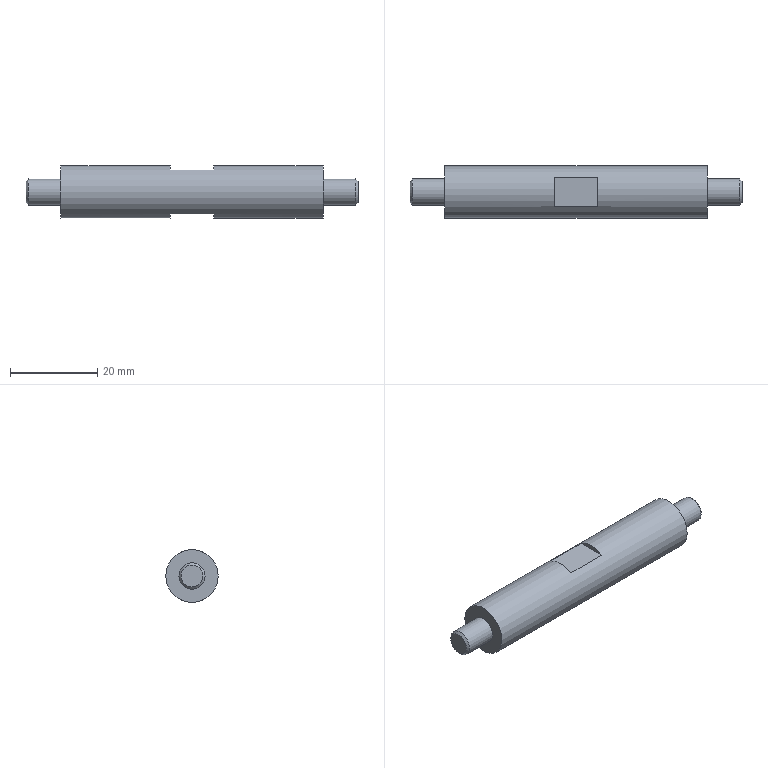Part | NX | features BREP 1 | 1 solid | 15 faces | box 76 x 12 x 12 mm | volume 7144 mm3 | plane 10 | cylinder 3 | cone 2 | commonest cylinder face diameters 6 x2 12 x1
STEP:
#1=CARTESIAN_POINT('',(30.,-6.,0.));
#2=VERTEX_POINT('',#1);
#3=CARTESIAN_POINT('',(30.,0.,0.));
#4=DIRECTION('',(-1.,0.,0.));
#5=DIRECTION('',(0.,-1.,0.));
#6=AXIS2_PLACEMENT_3D('',#3,#4,#5);
#7=CIRCLE('',#6,6.);
#8=EDGE_CURVE('',#2,#2,#7,.T.);
#9=ORIENTED_EDGE('',*,*,#8,.T.);
#10=EDGE_LOOP('',(#9));
#11=FACE_BOUND('',#10,.T.);
#12=CARTESIAN_POINT('',(-5.,-3.317,-5.));
#13=VERTEX_POINT('',#12);
#14=CARTESIAN_POINT('',(5.,-3.317,-5.));
#15=VERTEX_POINT('',#14);
#16=CARTESIAN_POINT('',(-38.,-3.317,-5.));
#17=DIRECTION('',(1.,0.,0.));
#18=VECTOR('',#17,1000.);
#19=LINE('',#16,#18);
#20=EDGE_CURVE('',#13,#15,#19,.T.);
#21=ORIENTED_EDGE('',*,*,#20,.T.);
#22=CARTESIAN_POINT('',(5.,3.317,-5.));
#23=VERTEX_POINT('',#22);
#24=CARTESIAN_POINT('',(5.,0.,0.));
#25=DIRECTION('',(1.,0.,0.));
#26=DIRECTION('',(0.,-1.,0.));
#27=AXIS2_PLACEMENT_3D('',#24,#25,#26);
#28=CIRCLE('',#27,6.);
#29=EDGE_CURVE('',#15,#23,#28,.T.);
#30=ORIENTED_EDGE('',*,*,#29,.T.);
#31=CARTESIAN_POINT('',(-5.,3.317,-5.));
#32=VERTEX_POINT('',#31);
#33=CARTESIAN_POINT('',(-38.,3.317,-5.));
#34=DIRECTION('',(-1.,0.,0.));
#35=VECTOR('',#34,1000.);
#36=LINE('',#33,#35);
#37=EDGE_CURVE('',#23,#32,#36,.T.);
#38=ORIENTED_EDGE('',*,*,#37,.T.);
#39=CARTESIAN_POINT('',(-5.,0.,0.));
#40=DIRECTION('',(-1.,0.,0.));
#41=DIRECTION('',(0.,-1.,0.));
#42=AXIS2_PLACEMENT_3D('',#39,#40,#41);
#43=CIRCLE('',#42,6.);
#44=EDGE_CURVE('',#32,#13,#43,.T.);
#45=ORIENTED_EDGE('',*,*,#44,.T.);
#46=EDGE_LOOP('',(#21,#30,#38,#45));
#47=FACE_BOUND('',#46,.T.);
#48=CARTESIAN_POINT('',(-30.,-6.,0.));
#49=VERTEX_POINT('',#48);
#50=CARTESIAN_POINT('',(-30.,0.,0.));
#51=DIRECTION('',(1.,0.,0.));
#52=DIRECTION('',(0.,-1.,0.));
#53=AXIS2_PLACEMENT_3D('',#50,#51,#52);
#54=CIRCLE('',#53,6.);
#55=EDGE_CURVE('',#49,#49,#54,.T.);
#56=ORIENTED_EDGE('',*,*,#55,.T.);
#57=EDGE_LOOP('',(#56));
#58=FACE_BOUND('',#57,.T.);
#59=CARTESIAN_POINT('',(5.,3.317,5.));
#60=VERTEX_POINT('',#59);
#61=CARTESIAN_POINT('',(5.,-3.317,5.));
#62=VERTEX_POINT('',#61);
#63=CARTESIAN_POINT('',(5.,0.,0.));
#64=DIRECTION('',(1.,0.,0.));
#65=DIRECTION('',(0.,-1.,0.));
#66=AXIS2_PLACEMENT_3D('',#63,#64,#65);
#67=CIRCLE('',#66,6.);
#68=EDGE_CURVE('',#60,#62,#67,.T.);
#69=ORIENTED_EDGE('',*,*,#68,.T.);
#70=CARTESIAN_POINT('',(-5.,-3.317,5.));
#71=VERTEX_POINT('',#70);
#72=CARTESIAN_POINT('',(-38.,-3.317,5.));
#73=DIRECTION('',(-1.,0.,0.));
#74=VECTOR('',#73,1000.);
#75=LINE('',#72,#74);
#76=EDGE_CURVE('',#62,#71,#75,.T.);
#77=ORIENTED_EDGE('',*,*,#76,.T.);
#78=CARTESIAN_POINT('',(-5.,3.317,5.));
#79=VERTEX_POINT('',#78);
#80=CARTESIAN_POINT('',(-5.,0.,0.));
#81=DIRECTION('',(-1.,0.,0.));
#82=DIRECTION('',(0.,-1.,0.));
#83=AXIS2_PLACEMENT_3D('',#80,#81,#82);
#84=CIRCLE('',#83,6.);
#85=EDGE_CURVE('',#71,#79,#84,.T.);
#86=ORIENTED_EDGE('',*,*,#85,.T.);
#87=CARTESIAN_POINT('',(-38.,3.317,5.));
#88=DIRECTION('',(1.,0.,0.));
#89=VECTOR('',#88,1000.);
#90=LINE('',#87,#89);
#91=EDGE_CURVE('',#79,#60,#90,.T.);
#92=ORIENTED_EDGE('',*,*,#91,.T.);
#93=EDGE_LOOP('',(#69,#77,#86,#92));
#94=FACE_BOUND('',#93,.T.);
#95=CARTESIAN_POINT('',(-38.,0.,0.));
#96=DIRECTION('',(-1.,0.,0.));
#97=DIRECTION('',(0.,1.,0.));
#98=AXIS2_PLACEMENT_3D('',#95,#96,#97);
#99=CYLINDRICAL_SURFACE('',#98,6.);
#100=ADVANCED_FACE('',(#11,#47,#58,#94),#99,.T.);
#101=ORIENTED_EDGE('',*,*,#29,.F.);
#102=CARTESIAN_POINT('',(5.,0.,-5.));
#103=DIRECTION('',(0.,1.,0.));
#104=VECTOR('',#103,1000.);
#105=LINE('',#102,#104);
#106=EDGE_CURVE('',#15,#23,#105,.T.);
#107=ORIENTED_EDGE('',*,*,#106,.T.);
#108=EDGE_LOOP('',(#101,#107));
#109=FACE_BOUND('',#108,.T.);
#110=CARTESIAN_POINT('',(5.,0.,0.));
#111=DIRECTION('',(-1.,0.,0.));
#112=DIRECTION('',(0.,0.,-1.));
#113=AXIS2_PLACEMENT_3D('',#110,#111,#112);
#114=PLANE('',#113);
#115=ADVANCED_FACE('',(#109),#114,.T.);
#116=ORIENTED_EDGE('',*,*,#20,.F.);
#117=CARTESIAN_POINT('',(-5.,6.286,-5.));
#118=DIRECTION('',(0.,-1.,0.));
#119=VECTOR('',#118,1000.);
#120=LINE('',#117,#119);
#121=EDGE_CURVE('',#32,#13,#120,.T.);
#122=ORIENTED_EDGE('',*,*,#121,.F.);
#123=ORIENTED_EDGE('',*,*,#37,.F.);
#124=ORIENTED_EDGE('',*,*,#106,.F.);
#125=EDGE_LOOP('',(#116,#122,#123,#124));
#126=FACE_BOUND('',#125,.T.);
#127=CARTESIAN_POINT('',(-5.,6.286,-5.));
#128=DIRECTION('',(0.,0.,1.));
#129=DIRECTION('',(-1.,0.,0.));
#130=AXIS2_PLACEMENT_3D('',#127,#128,#129);
#131=PLANE('',#130);
#132=ADVANCED_FACE('',(#126),#131,.F.);
#133=ORIENTED_EDGE('',*,*,#44,.F.);
#134=ORIENTED_EDGE('',*,*,#121,.T.);
#135=EDGE_LOOP('',(#133,#134));
#136=FACE_BOUND('',#135,.T.);
#137=CARTESIAN_POINT('',(-5.,0.,0.));
#138=DIRECTION('',(-1.,0.,0.));
#139=DIRECTION('',(0.,0.,-1.));
#140=AXIS2_PLACEMENT_3D('',#137,#138,#139);
#141=PLANE('',#140);
#142=ADVANCED_FACE('',(#136),#141,.F.);
#143=ORIENTED_EDGE('',*,*,#55,.F.);
#144=EDGE_LOOP('',(#143));
#145=FACE_BOUND('',#144,.T.);
#146=CARTESIAN_POINT('',(-30.,-3.,0.));
#147=VERTEX_POINT('',#146);
#148=CARTESIAN_POINT('',(-30.,0.,0.));
#149=DIRECTION('',(-1.,0.,0.));
#150=DIRECTION('',(0.,-1.,0.));
#151=AXIS2_PLACEMENT_3D('',#148,#149,#150);
#152=CIRCLE('',#151,3.);
#153=EDGE_CURVE('',#147,#147,#152,.T.);
#154=ORIENTED_EDGE('',*,*,#153,.F.);
#155=EDGE_LOOP('',(#154));
#156=FACE_BOUND('',#155,.T.);
#157=CARTESIAN_POINT('',(-30.,6.,0.));
#158=DIRECTION('',(1.,0.,0.));
#159=DIRECTION('',(0.,-1.,0.));
#160=AXIS2_PLACEMENT_3D('',#157,#158,#159);
#161=PLANE('',#160);
#162=ADVANCED_FACE('',(#145,#156),#161,.F.);
#163=CARTESIAN_POINT('',(30.,-3.,0.));
#164=VERTEX_POINT('',#163);
#165=CARTESIAN_POINT('',(30.,0.,0.));
#166=DIRECTION('',(1.,0.,0.));
#167=DIRECTION('',(0.,-1.,0.));
#168=AXIS2_PLACEMENT_3D('',#165,#166,#167);
#169=CIRCLE('',#168,3.);
#170=EDGE_CURVE('',#164,#164,#169,.T.);
#171=ORIENTED_EDGE('',*,*,#170,.F.);
#172=EDGE_LOOP('',(#171));
#173=FACE_BOUND('',#172,.T.);
#174=ORIENTED_EDGE('',*,*,#8,.F.);
#175=EDGE_LOOP('',(#174));
#176=FACE_BOUND('',#175,.T.);
#177=CARTESIAN_POINT('',(30.,3.,0.));
#178=DIRECTION('',(-1.,0.,0.));
#179=DIRECTION('',(0.,1.,0.));
#180=AXIS2_PLACEMENT_3D('',#177,#178,#179);
#181=PLANE('',#180);
#182=ADVANCED_FACE('',(#173,#176),#181,.F.);
#183=CARTESIAN_POINT('',(-37.5,-3.,0.));
#184=VERTEX_POINT('',#183);
#185=CARTESIAN_POINT('',(-37.5,0.,0.));
#186=DIRECTION('',(1.,0.,0.));
#187=DIRECTION('',(0.,-1.,0.));
#188=AXIS2_PLACEMENT_3D('',#185,#186,#187);
#189=CIRCLE('',#188,3.);
#190=EDGE_CURVE('',#184,#184,#189,.T.);
#191=ORIENTED_EDGE('',*,*,#190,.T.);
#192=EDGE_LOOP('',(#191));
#193=FACE_BOUND('',#192,.T.);
#194=ORIENTED_EDGE('',*,*,#153,.T.);
#195=EDGE_LOOP('',(#194));
#196=FACE_BOUND('',#195,.T.);
#197=CARTESIAN_POINT('',(-38.,0.,0.));
#198=DIRECTION('',(-1.,0.,0.));
#199=DIRECTION('',(0.,1.,0.));
#200=AXIS2_PLACEMENT_3D('',#197,#198,#199);
#201=CYLINDRICAL_SURFACE('',#200,3.);
#202=ADVANCED_FACE('',(#193,#196),#201,.T.);
#203=ORIENTED_EDGE('',*,*,#91,.F.);
#204=CARTESIAN_POINT('',(-5.,6.286,5.));
#205=DIRECTION('',(0.,1.,0.));
#206=VECTOR('',#205,1000.);
#207=LINE('',#204,#206);
#208=EDGE_CURVE('',#71,#79,#207,.T.);
#209=ORIENTED_EDGE('',*,*,#208,.F.);
#210=ORIENTED_EDGE('',*,*,#76,.F.);
#211=CARTESIAN_POINT('',(5.,6.286,5.));
#212=DIRECTION('',(0.,-1.,0.));
#213=VECTOR('',#212,1000.);
#214=LINE('',#211,#213);
#215=EDGE_CURVE('',#60,#62,#214,.T.);
#216=ORIENTED_EDGE('',*,*,#215,.F.);
#217=EDGE_LOOP('',(#203,#209,#210,#216));
#218=FACE_BOUND('',#217,.T.);
#219=CARTESIAN_POINT('',(-5.,6.286,5.));
#220=DIRECTION('',(0.,0.,-1.));
#221=DIRECTION('',(1.,0.,0.));
#222=AXIS2_PLACEMENT_3D('',#219,#220,#221);
#223=PLANE('',#222);
#224=ADVANCED_FACE('',(#218),#223,.F.);
#225=ORIENTED_EDGE('',*,*,#68,.F.);
#226=ORIENTED_EDGE('',*,*,#215,.T.);
#227=EDGE_LOOP('',(#225,#226));
#228=FACE_BOUND('',#227,.T.);
#229=CARTESIAN_POINT('',(5.,0.,0.));
#230=DIRECTION('',(1.,0.,0.));
#231=DIRECTION('',(0.,0.,1.));
#232=AXIS2_PLACEMENT_3D('',#229,#230,#231);
#233=PLANE('',#232);
#234=ADVANCED_FACE('',(#228),#233,.F.);
#235=ORIENTED_EDGE('',*,*,#85,.F.);
#236=ORIENTED_EDGE('',*,*,#208,.T.);
#237=EDGE_LOOP('',(#235,#236));
#238=FACE_BOUND('',#237,.T.);
#239=CARTESIAN_POINT('',(-5.,0.,0.));
#240=DIRECTION('',(1.,0.,0.));
#241=DIRECTION('',(0.,0.,1.));
#242=AXIS2_PLACEMENT_3D('',#239,#240,#241);
#243=PLANE('',#242);
#244=ADVANCED_FACE('',(#238),#243,.T.);
#245=ORIENTED_EDGE('',*,*,#170,.T.);
#246=EDGE_LOOP('',(#245));
#247=FACE_BOUND('',#246,.T.);
#248=CARTESIAN_POINT('',(37.5,-3.,0.));
#249=VERTEX_POINT('',#248);
#250=CARTESIAN_POINT('',(37.5,0.,0.));
#251=DIRECTION('',(-1.,0.,0.));
#252=DIRECTION('',(0.,-1.,0.));
#253=AXIS2_PLACEMENT_3D('',#250,#251,#252);
#254=CIRCLE('',#253,3.);
#255=EDGE_CURVE('',#249,#249,#254,.T.);
#256=ORIENTED_EDGE('',*,*,#255,.T.);
#257=EDGE_LOOP('',(#256));
#258=FACE_BOUND('',#257,.T.);
#259=CARTESIAN_POINT('',(-38.,0.,0.));
#260=DIRECTION('',(-1.,0.,0.));
#261=DIRECTION('',(0.,1.,0.));
#262=AXIS2_PLACEMENT_3D('',#259,#260,#261);
#263=CYLINDRICAL_SURFACE('',#262,3.);
#264=ADVANCED_FACE('',(#247,#258),#263,.T.);
#265=ORIENTED_EDGE('',*,*,#190,.F.);
#266=EDGE_LOOP('',(#265));
#267=FACE_BOUND('',#266,.T.);
#268=CARTESIAN_POINT('',(-38.,0.,-2.5));
#269=VERTEX_POINT('',#268);
#270=CARTESIAN_POINT('',(-38.,0.,0.));
#271=DIRECTION('',(1.,0.,0.));
#272=DIRECTION('',(0.,0.,-1.));
#273=AXIS2_PLACEMENT_3D('',#270,#271,#272);
#274=CIRCLE('',#273,2.5);
#275=EDGE_CURVE('',#269,#269,#274,.T.);
#276=ORIENTED_EDGE('',*,*,#275,.T.);
#277=EDGE_LOOP('',(#276));
#278=FACE_BOUND('',#277,.T.);
#279=CARTESIAN_POINT('',(-37.5,0.,0.));
#280=DIRECTION('',(1.,0.,0.));
#281=DIRECTION('',(0.,0.,1.));
#282=AXIS2_PLACEMENT_3D('',#279,#280,#281);
#283=CONICAL_SURFACE('',#282,3.,0.7854);
#284=ADVANCED_FACE('',(#267,#278),#283,.T.);
#285=ORIENTED_EDGE('',*,*,#255,.F.);
#286=EDGE_LOOP('',(#285));
#287=FACE_BOUND('',#286,.T.);
#288=CARTESIAN_POINT('',(38.,0.,2.5));
#289=VERTEX_POINT('',#288);
#290=CARTESIAN_POINT('',(38.,0.,0.));
#291=DIRECTION('',(-1.,0.,0.));
#292=DIRECTION('',(0.,0.,1.));
#293=AXIS2_PLACEMENT_3D('',#290,#291,#292);
#294=CIRCLE('',#293,2.5);
#295=EDGE_CURVE('',#289,#289,#294,.T.);
#296=ORIENTED_EDGE('',*,*,#295,.T.);
#297=EDGE_LOOP('',(#296));
#298=FACE_BOUND('',#297,.T.);
#299=CARTESIAN_POINT('',(37.5,0.,0.));
#300=DIRECTION('',(-1.,0.,0.));
#301=DIRECTION('',(0.,0.,-1.));
#302=AXIS2_PLACEMENT_3D('',#299,#300,#301);
#303=CONICAL_SURFACE('',#302,3.,0.7854);
#304=ADVANCED_FACE('',(#287,#298),#303,.T.);
#305=ORIENTED_EDGE('',*,*,#275,.F.);
#306=EDGE_LOOP('',(#305));
#307=FACE_BOUND('',#306,.T.);
#308=CARTESIAN_POINT('',(-38.,3.,0.));
#309=DIRECTION('',(1.,0.,0.));
#310=DIRECTION('',(0.,-1.,0.));
#311=AXIS2_PLACEMENT_3D('',#308,#309,#310);
#312=PLANE('',#311);
#313=ADVANCED_FACE('',(#307),#312,.F.);
#314=ORIENTED_EDGE('',*,*,#295,.F.);
#315=EDGE_LOOP('',(#314));
#316=FACE_BOUND('',#315,.T.);
#317=CARTESIAN_POINT('',(38.,0.,0.));
#318=DIRECTION('',(-1.,0.,0.));
#319=DIRECTION('',(0.,1.,0.));
#320=AXIS2_PLACEMENT_3D('',#317,#318,#319);
#321=PLANE('',#320);
#322=ADVANCED_FACE('',(#316),#321,.F.);
#323=CLOSED_SHELL('',(#100,#115,#132,#142,#162,#182,#202,#224,#234,#244,#264,#284,#304,#313,#322));
#324=MANIFOLD_SOLID_BREP('',#323);
#325=(LENGTH_UNIT()NAMED_UNIT(*)SI_UNIT(.MILLI.,.METRE.));
#326=UNCERTAINTY_MEASURE_WITH_UNIT(LENGTH_MEASURE(0.00001),#325,'','');
#327=(NAMED_UNIT(*)PLANE_ANGLE_UNIT()SI_UNIT($,.RADIAN.));
#328=(NAMED_UNIT(*)SI_UNIT($,.STERADIAN.)SOLID_ANGLE_UNIT());
#329=(GEOMETRIC_REPRESENTATION_CONTEXT(3)GLOBAL_UNCERTAINTY_ASSIGNED_CONTEXT((#326))GLOBAL_UNIT_ASSIGNED_CONTEXT((#325,#327,#328))REPRESENTATION_CONTEXT('',''));
#330=ADVANCED_BREP_SHAPE_REPRESENTATION('',(#324),#329);